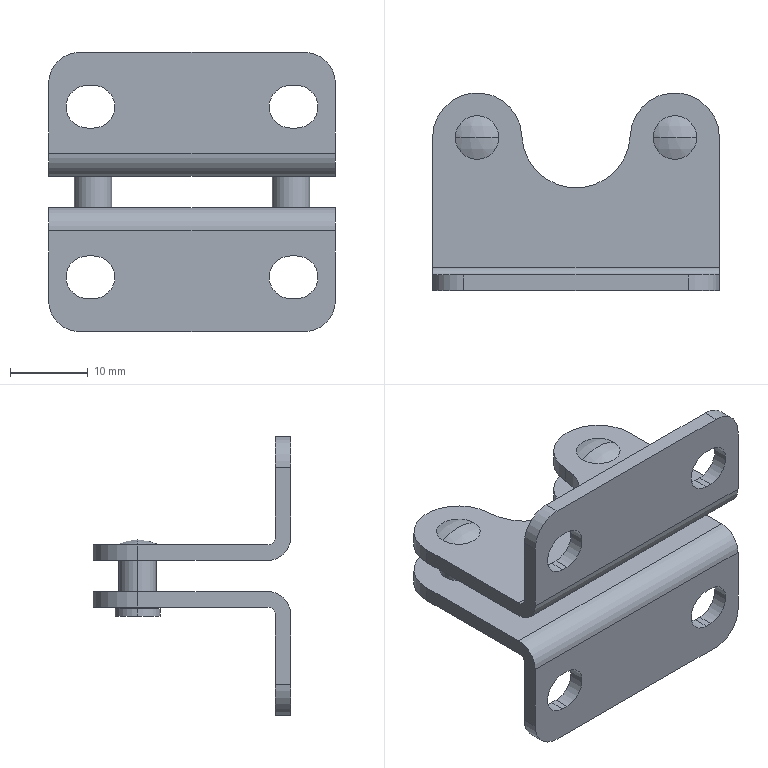Part | STEP file | 11-BASE_MC01-S311 | 1 solid | 64 faces | box 37 x 25.5 x 36 mm | volume 4977 mm3 | cylinder 34 | plane 26 | sphere 4 | commonest cylinder face diameters 4.85 x8 5.5 x8 5.85 x4 8 x4 11.5 x4 2 x2